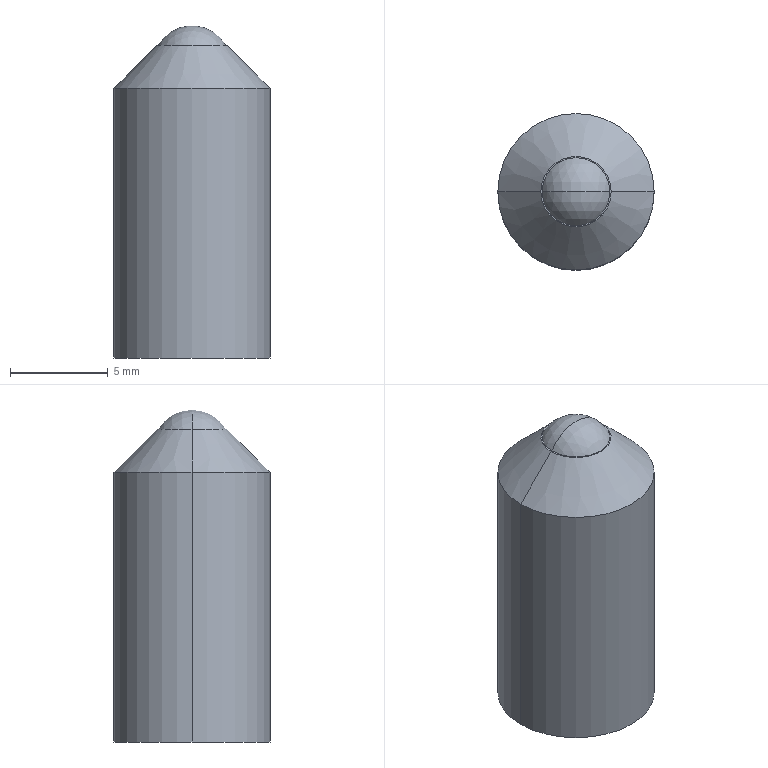Part | SolidWorks | features Chamfer 1, Extrusion 1, Revolution 1 | 1 solid | 8 faces | box 8 x 8 x 17 mm | volume 759.813 mm3 | cone 2 | sphere 2 | cylinder 2 | plane 2 | commonest cylinder face diameters 8 x2
STEP:
#1=CARTESIAN_POINT('',(1.8,0.,16.));
#2=VERTEX_POINT('',#1);
#3=CARTESIAN_POINT('',(-1.8,0.,16.));
#4=VERTEX_POINT('',#3);
#5=CARTESIAN_POINT('',(0.,0.,16.));
#6=DIRECTION('',(0.,0.,1.));
#7=DIRECTION('',(1.,0.,0.));
#8=AXIS2_PLACEMENT_3D('',#5,#6,#7);
#9=CIRCLE('',#8,1.8);
#10=EDGE_CURVE('',#2,#4,#9,.T.);
#11=ORIENTED_EDGE('',*,*,#10,.F.);
#12=CARTESIAN_POINT('',(4.,0.,13.8));
#13=VERTEX_POINT('',#12);
#14=CARTESIAN_POINT('',(1.8,0.,16.));
#15=DIRECTION('',(0.7071,0.,-0.7071));
#16=VECTOR('',#15,1000.);
#17=LINE('',#14,#16);
#18=EDGE_CURVE('',#2,#13,#17,.T.);
#19=ORIENTED_EDGE('',*,*,#18,.T.);
#20=CARTESIAN_POINT('',(-4.,0.,13.8));
#21=VERTEX_POINT('',#20);
#22=CARTESIAN_POINT('',(0.,0.,13.8));
#23=DIRECTION('',(0.,0.,-1.));
#24=DIRECTION('',(1.,0.,0.));
#25=AXIS2_PLACEMENT_3D('',#22,#23,#24);
#26=CIRCLE('',#25,4.);
#27=EDGE_CURVE('',#21,#13,#26,.T.);
#28=ORIENTED_EDGE('',*,*,#27,.F.);
#29=CARTESIAN_POINT('',(-1.8,0.,16.));
#30=DIRECTION('',(-0.7071,0.,-0.7071));
#31=VECTOR('',#30,1000.);
#32=LINE('',#29,#31);
#33=EDGE_CURVE('',#4,#21,#32,.T.);
#34=ORIENTED_EDGE('',*,*,#33,.F.);
#35=EDGE_LOOP('',(#11,#19,#28,#34));
#36=FACE_OUTER_BOUND('',#35,.T.);
#37=CARTESIAN_POINT('',(0.,0.,16.));
#38=DIRECTION('',(0.,0.,-1.));
#39=DIRECTION('',(-1.,0.,0.));
#40=AXIS2_PLACEMENT_3D('',#37,#38,#39);
#41=CONICAL_SURFACE('',#40,1.8,0.7854);
#42=ADVANCED_FACE('',(#36),#41,.T.);
#43=CARTESIAN_POINT('',(-1.732,0.,16.));
#44=VERTEX_POINT('',#43);
#45=CARTESIAN_POINT('',(1.732,0.,16.));
#46=VERTEX_POINT('',#45);
#47=CARTESIAN_POINT('',(0.,0.,16.));
#48=DIRECTION('',(0.,0.,1.));
#49=DIRECTION('',(1.,0.,0.));
#50=AXIS2_PLACEMENT_3D('',#47,#48,#49);
#51=CIRCLE('',#50,1.732);
#52=EDGE_CURVE('',#44,#46,#51,.T.);
#53=ORIENTED_EDGE('',*,*,#52,.T.);
#54=CARTESIAN_POINT('',(0.,0.,15.));
#55=DIRECTION('',(0.,-1.,0.));
#56=DIRECTION('',(0.,0.,-1.));
#57=AXIS2_PLACEMENT_3D('',#54,#55,#56);
#58=CIRCLE('',#57,2.);
#59=EDGE_CURVE('',#46,#44,#58,.T.);
#60=ORIENTED_EDGE('',*,*,#59,.T.);
#61=EDGE_LOOP('',(#53,#60));
#62=FACE_OUTER_BOUND('',#61,.T.);
#63=CARTESIAN_POINT('',(0.,0.,15.));
#64=DIRECTION('',(0.,-1.,0.));
#65=DIRECTION('',(0.,0.,-1.));
#66=AXIS2_PLACEMENT_3D('',#63,#64,#65);
#67=SPHERICAL_SURFACE('',#66,2.);
#68=ADVANCED_FACE('',(#62),#67,.T.);
#69=ORIENTED_EDGE('',*,*,#27,.T.);
#70=CARTESIAN_POINT('',(4.,0.,0.));
#71=VERTEX_POINT('',#70);
#72=CARTESIAN_POINT('',(4.,0.,16.));
#73=DIRECTION('',(0.,0.,-1.));
#74=VECTOR('',#73,1000.);
#75=LINE('',#72,#74);
#76=EDGE_CURVE('',#13,#71,#75,.T.);
#77=ORIENTED_EDGE('',*,*,#76,.T.);
#78=CARTESIAN_POINT('',(-4.,0.,0.));
#79=VERTEX_POINT('',#78);
#80=CARTESIAN_POINT('',(0.,0.,0.));
#81=DIRECTION('',(0.,0.,1.));
#82=DIRECTION('',(1.,0.,0.));
#83=AXIS2_PLACEMENT_3D('',#80,#81,#82);
#84=CIRCLE('',#83,4.);
#85=EDGE_CURVE('',#71,#79,#84,.T.);
#86=ORIENTED_EDGE('',*,*,#85,.T.);
#87=CARTESIAN_POINT('',(-4.,0.,16.));
#88=DIRECTION('',(0.,0.,-1.));
#89=VECTOR('',#88,1000.);
#90=LINE('',#87,#89);
#91=EDGE_CURVE('',#21,#79,#90,.T.);
#92=ORIENTED_EDGE('',*,*,#91,.F.);
#93=EDGE_LOOP('',(#69,#77,#86,#92));
#94=FACE_OUTER_BOUND('',#93,.T.);
#95=CARTESIAN_POINT('',(0.,0.,16.));
#96=DIRECTION('',(0.,0.,-1.));
#97=DIRECTION('',(-1.,0.,0.));
#98=AXIS2_PLACEMENT_3D('',#95,#96,#97);
#99=CYLINDRICAL_SURFACE('',#98,4.);
#100=ADVANCED_FACE('',(#94),#99,.T.);
#101=ORIENTED_EDGE('',*,*,#76,.F.);
#102=CARTESIAN_POINT('',(0.,0.,13.8));
#103=DIRECTION('',(0.,0.,-1.));
#104=DIRECTION('',(1.,0.,0.));
#105=AXIS2_PLACEMENT_3D('',#102,#103,#104);
#106=CIRCLE('',#105,4.);
#107=EDGE_CURVE('',#13,#21,#106,.T.);
#108=ORIENTED_EDGE('',*,*,#107,.T.);
#109=ORIENTED_EDGE('',*,*,#91,.T.);
#110=CARTESIAN_POINT('',(0.,0.,0.));
#111=DIRECTION('',(0.,0.,1.));
#112=DIRECTION('',(1.,0.,0.));
#113=AXIS2_PLACEMENT_3D('',#110,#111,#112);
#114=CIRCLE('',#113,4.);
#115=EDGE_CURVE('',#79,#71,#114,.T.);
#116=ORIENTED_EDGE('',*,*,#115,.T.);
#117=EDGE_LOOP('',(#101,#108,#109,#116));
#118=FACE_OUTER_BOUND('',#117,.T.);
#119=CARTESIAN_POINT('',(0.,0.,16.));
#120=DIRECTION('',(0.,0.,-1.));
#121=DIRECTION('',(-1.,0.,0.));
#122=AXIS2_PLACEMENT_3D('',#119,#120,#121);
#123=CYLINDRICAL_SURFACE('',#122,4.);
#124=ADVANCED_FACE('',(#118),#123,.T.);
#125=CARTESIAN_POINT('',(0.,0.,16.));
#126=DIRECTION('',(0.,0.,1.));
#127=DIRECTION('',(1.,0.,0.));
#128=AXIS2_PLACEMENT_3D('',#125,#126,#127);
#129=CIRCLE('',#128,1.8);
#130=EDGE_CURVE('',#4,#2,#129,.T.);
#131=ORIENTED_EDGE('',*,*,#130,.T.);
#132=ORIENTED_EDGE('',*,*,#10,.T.);
#133=EDGE_LOOP('',(#131,#132));
#134=FACE_OUTER_BOUND('',#133,.T.);
#135=CARTESIAN_POINT('',(0.,0.,16.));
#136=DIRECTION('',(0.,0.,1.));
#137=DIRECTION('',(1.,0.,0.));
#138=AXIS2_PLACEMENT_3D('',#135,#136,#137);
#139=CIRCLE('',#138,1.732);
#140=EDGE_CURVE('',#46,#44,#139,.T.);
#141=ORIENTED_EDGE('',*,*,#140,.F.);
#142=ORIENTED_EDGE('',*,*,#52,.F.);
#143=EDGE_LOOP('',(#141,#142));
#144=FACE_BOUND('',#143,.T.);
#145=CARTESIAN_POINT('',(0.,0.,16.));
#146=DIRECTION('',(0.,0.,1.));
#147=DIRECTION('',(1.,0.,0.));
#148=AXIS2_PLACEMENT_3D('',#145,#146,#147);
#149=PLANE('',#148);
#150=ADVANCED_FACE('',(#134,#144),#149,.T.);
#151=ORIENTED_EDGE('',*,*,#115,.F.);
#152=ORIENTED_EDGE('',*,*,#85,.F.);
#153=EDGE_LOOP('',(#151,#152));
#154=FACE_OUTER_BOUND('',#153,.T.);
#155=CARTESIAN_POINT('',(0.,0.,0.));
#156=DIRECTION('',(0.,0.,1.));
#157=DIRECTION('',(1.,0.,0.));
#158=AXIS2_PLACEMENT_3D('',#155,#156,#157);
#159=PLANE('',#158);
#160=ADVANCED_FACE('',(#154),#159,.F.);
#161=ORIENTED_EDGE('',*,*,#59,.F.);
#162=ORIENTED_EDGE('',*,*,#140,.T.);
#163=EDGE_LOOP('',(#161,#162));
#164=FACE_OUTER_BOUND('',#163,.T.);
#165=CARTESIAN_POINT('',(0.,0.,15.));
#166=DIRECTION('',(0.,-1.,0.));
#167=DIRECTION('',(0.,0.,-1.));
#168=AXIS2_PLACEMENT_3D('',#165,#166,#167);
#169=SPHERICAL_SURFACE('',#168,2.);
#170=ADVANCED_FACE('',(#164),#169,.T.);
#171=ORIENTED_EDGE('',*,*,#18,.F.);
#172=ORIENTED_EDGE('',*,*,#130,.F.);
#173=ORIENTED_EDGE('',*,*,#33,.T.);
#174=ORIENTED_EDGE('',*,*,#107,.F.);
#175=EDGE_LOOP('',(#171,#172,#173,#174));
#176=FACE_OUTER_BOUND('',#175,.T.);
#177=CARTESIAN_POINT('',(0.,0.,16.));
#178=DIRECTION('',(0.,0.,-1.));
#179=DIRECTION('',(-1.,0.,0.));
#180=AXIS2_PLACEMENT_3D('',#177,#178,#179);
#181=CONICAL_SURFACE('',#180,1.8,0.7854);
#182=ADVANCED_FACE('',(#176),#181,.T.);
#183=CLOSED_SHELL('',(#42,#68,#100,#124,#150,#160,#170,#182));
#184=MANIFOLD_SOLID_BREP('',#183);
#185=CARTESIAN_POINT('',(0.,0.,0.));
#186=DIRECTION('',(0.,0.,1.));
#187=DIRECTION('',(1.,0.,0.));
#188=AXIS2_PLACEMENT_3D('',#185,#186,#187);
#189=(LENGTH_UNIT()NAMED_UNIT(*)SI_UNIT(.MILLI.,.METRE.));
#190=UNCERTAINTY_MEASURE_WITH_UNIT(LENGTH_MEASURE(0.00001),#189,'','');
#191=(NAMED_UNIT(*)PLANE_ANGLE_UNIT()SI_UNIT($,.RADIAN.));
#192=(NAMED_UNIT(*)SI_UNIT($,.STERADIAN.)SOLID_ANGLE_UNIT());
#193=(GEOMETRIC_REPRESENTATION_CONTEXT(3)GLOBAL_UNCERTAINTY_ASSIGNED_CONTEXT((#190))GLOBAL_UNIT_ASSIGNED_CONTEXT((#189,#191,#192))REPRESENTATION_CONTEXT('',''));
#194=ADVANCED_BREP_SHAPE_REPRESENTATION('',(#184,#188),#193);